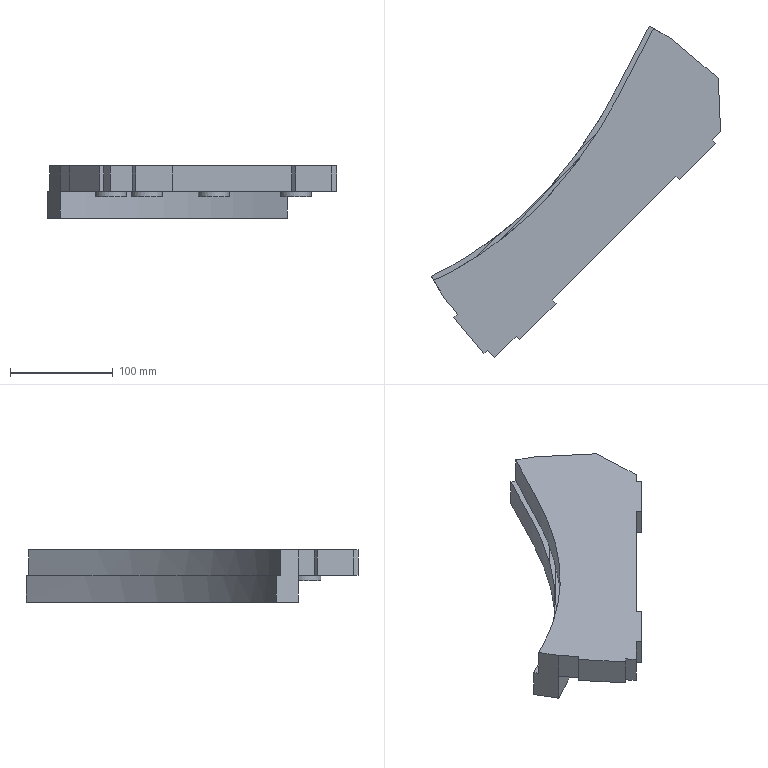Part | NX | features solid 2 | 1 solid | 38 faces | box 281.55 x 323.19 x 51 mm | volume 976674 mm3 | plane 29 | cylinder 5 | spline 4 | commonest cylinder face diameters 30 x5
STEP:
#1=CARTESIAN_POINT('',(378.604,-622.777,20.));
#2=VERTEX_POINT('',#1);
#3=CARTESIAN_POINT('',(378.604,-622.777,45.));
#4=VERTEX_POINT('',#3);
#5=CARTESIAN_POINT('',(378.604,-622.777,20.));
#6=DIRECTION('',(0.,0.,1.));
#7=VECTOR('',#6,1000.);
#8=LINE('',#5,#7);
#9=EDGE_CURVE('',#2,#4,#8,.T.);
#10=ORIENTED_EDGE('',*,*,#9,.F.);
#11=CARTESIAN_POINT('',(385.032,-630.437,20.));
#12=VERTEX_POINT('',#11);
#13=CARTESIAN_POINT('',(339.027,-575.611,20.));
#14=DIRECTION('',(-0.6428,0.766,0.));
#15=VECTOR('',#14,1000.);
#16=LINE('',#13,#15);
#17=EDGE_CURVE('',#12,#2,#16,.T.);
#18=ORIENTED_EDGE('',*,*,#17,.F.);
#19=CARTESIAN_POINT('',(385.032,-630.437,45.));
#20=VERTEX_POINT('',#19);
#21=CARTESIAN_POINT('',(385.032,-630.437,45.));
#22=DIRECTION('',(0.,0.,1.));
#23=VECTOR('',#22,1000.);
#24=LINE('',#21,#23);
#25=EDGE_CURVE('',#12,#20,#24,.T.);
#26=ORIENTED_EDGE('',*,*,#25,.T.);
#27=CARTESIAN_POINT('',(323.293,-556.86,45.));
#28=DIRECTION('',(0.6428,-0.766,0.));
#29=VECTOR('',#28,1000.);
#30=LINE('',#27,#29);
#31=EDGE_CURVE('',#4,#20,#30,.T.);
#32=ORIENTED_EDGE('',*,*,#31,.F.);
#33=EDGE_LOOP('',(#10,#18,#26,#32));
#34=FACE_BOUND('',#33,.T.);
#35=CARTESIAN_POINT('',(389.886,-636.222,20.));
#36=DIRECTION('',(0.766,0.6428,0.));
#37=DIRECTION('',(-0.6428,0.766,0.));
#38=AXIS2_PLACEMENT_3D('',#35,#36,#37);
#39=PLANE('',#38);
#40=ADVANCED_FACE('',(#34),#39,.F.);
#41=CARTESIAN_POINT('',(349.161,-587.688,45.));
#42=VERTEX_POINT('',#41);
#43=CARTESIAN_POINT('',(349.161,-587.688,20.));
#44=VERTEX_POINT('',#43);
#45=CARTESIAN_POINT('',(349.161,-587.688,20.));
#46=DIRECTION('',(0.,0.,-1.));
#47=VECTOR('',#46,1000.);
#48=LINE('',#45,#47);
#49=EDGE_CURVE('',#42,#44,#48,.T.);
#50=ORIENTED_EDGE('',*,*,#49,.F.);
#51=CARTESIAN_POINT('',(336.306,-572.367,45.));
#52=VERTEX_POINT('',#51);
#53=CARTESIAN_POINT('',(323.293,-556.86,45.));
#54=DIRECTION('',(0.6428,-0.766,0.));
#55=VECTOR('',#54,1000.);
#56=LINE('',#53,#55);
#57=EDGE_CURVE('',#52,#42,#56,.T.);
#58=ORIENTED_EDGE('',*,*,#57,.F.);
#59=CARTESIAN_POINT('',(336.306,-572.367,20.));
#60=VERTEX_POINT('',#59);
#61=CARTESIAN_POINT('',(336.306,-572.367,45.));
#62=DIRECTION('',(0.,0.,-1.));
#63=VECTOR('',#62,1000.);
#64=LINE('',#61,#63);
#65=EDGE_CURVE('',#52,#60,#64,.T.);
#66=ORIENTED_EDGE('',*,*,#65,.T.);
#67=CARTESIAN_POINT('',(339.027,-575.611,20.));
#68=DIRECTION('',(-0.6428,0.766,0.));
#69=VECTOR('',#68,1000.);
#70=LINE('',#67,#69);
#71=EDGE_CURVE('',#44,#60,#70,.T.);
#72=ORIENTED_EDGE('',*,*,#71,.F.);
#73=EDGE_LOOP('',(#50,#58,#66,#72));
#74=FACE_BOUND('',#73,.T.);
#75=CARTESIAN_POINT('',(389.886,-636.222,20.));
#76=DIRECTION('',(0.766,0.6428,0.));
#77=DIRECTION('',(-0.6428,0.766,0.));
#78=AXIS2_PLACEMENT_3D('',#75,#76,#77);
#79=PLANE('',#78);
#80=ADVANCED_FACE('',(#74),#79,.F.);
#81=CARTESIAN_POINT('',(445.136,-577.404,20.));
#82=VERTEX_POINT('',#81);
#83=CARTESIAN_POINT('',(441.601,-573.869,20.));
#84=VERTEX_POINT('',#83);
#85=CARTESIAN_POINT('',(445.136,-577.404,20.));
#86=DIRECTION('',(-0.7071,0.7071,0.));
#87=VECTOR('',#86,1000.);
#88=LINE('',#85,#87);
#89=EDGE_CURVE('',#82,#84,#88,.T.);
#90=ORIENTED_EDGE('',*,*,#89,.F.);
#91=CARTESIAN_POINT('',(409.781,-612.76,20.));
#92=VERTEX_POINT('',#91);
#93=CARTESIAN_POINT('',(649.557,-372.983,20.));
#94=DIRECTION('',(-0.7071,-0.7071,0.));
#95=VECTOR('',#94,1000.);
#96=LINE('',#93,#95);
#97=EDGE_CURVE('',#82,#92,#96,.T.);
#98=ORIENTED_EDGE('',*,*,#97,.T.);
#99=CARTESIAN_POINT('',(406.245,-609.224,20.));
#100=VERTEX_POINT('',#99);
#101=CARTESIAN_POINT('',(409.781,-612.76,20.));
#102=DIRECTION('',(-0.7071,0.7071,0.));
#103=VECTOR('',#102,1000.);
#104=LINE('',#101,#103);
#105=EDGE_CURVE('',#92,#100,#104,.T.);
#106=ORIENTED_EDGE('',*,*,#105,.T.);
#107=CARTESIAN_POINT('',(646.022,-369.447,20.));
#108=DIRECTION('',(-0.7071,-0.7071,0.));
#109=VECTOR('',#108,1000.);
#110=LINE('',#107,#109);
#111=EDGE_CURVE('',#100,#12,#110,.T.);
#112=ORIENTED_EDGE('',*,*,#111,.T.);
#113=ORIENTED_EDGE('',*,*,#17,.T.);
#114=CARTESIAN_POINT('',(374.774,-625.991,20.));
#115=VERTEX_POINT('',#114);
#116=CARTESIAN_POINT('',(374.774,-625.991,20.));
#117=DIRECTION('',(0.766,0.6428,0.));
#118=VECTOR('',#117,1000.);
#119=LINE('',#116,#118);
#120=EDGE_CURVE('',#115,#2,#119,.T.);
#121=ORIENTED_EDGE('',*,*,#120,.F.);
#122=CARTESIAN_POINT('',(345.331,-590.902,20.));
#123=VERTEX_POINT('',#122);
#124=CARTESIAN_POINT('',(335.197,-578.825,20.));
#125=DIRECTION('',(-0.6428,0.766,0.));
#126=VECTOR('',#125,1000.);
#127=LINE('',#124,#126);
#128=EDGE_CURVE('',#115,#123,#127,.T.);
#129=ORIENTED_EDGE('',*,*,#128,.T.);
#130=CARTESIAN_POINT('',(345.331,-590.902,20.));
#131=DIRECTION('',(0.766,0.6428,0.));
#132=VECTOR('',#131,1000.);
#133=LINE('',#130,#132);
#134=EDGE_CURVE('',#123,#44,#133,.T.);
#135=ORIENTED_EDGE('',*,*,#134,.T.);
#136=ORIENTED_EDGE('',*,*,#71,.T.);
#137=CARTESIAN_POINT('',(557.374,-319.761,20.));
#138=VERTEX_POINT('',#137);
#139=CARTESIAN_POINT('',(557.374,-319.761,20.));
#140=CARTESIAN_POINT('',(551.234,-331.629,20.));
#141=CARTESIAN_POINT('',(541.911,-349.627,20.));
#142=CARTESIAN_POINT('',(531.108,-370.579,20.));
#143=CARTESIAN_POINT('',(524.631,-383.018,20.));
#144=CARTESIAN_POINT('',(514.348,-402.01,20.));
#145=CARTESIAN_POINT('',(497.659,-429.783,20.));
#146=CARTESIAN_POINT('',(471.931,-465.101,20.));
#147=CARTESIAN_POINT('',(442.6,-497.853,20.));
#148=CARTESIAN_POINT('',(409.743,-527.289,20.));
#149=CARTESIAN_POINT('',(379.681,-548.594,20.));
#150=CARTESIAN_POINT('',(357.354,-561.599,20.));
#151=CARTESIAN_POINT('',(346.037,-567.559,20.));
#152=CARTESIAN_POINT('',(339.912,-570.613,20.));
#153=CARTESIAN_POINT('',(337.327,-571.87,20.));
#154=CARTESIAN_POINT('',(336.306,-572.367,20.));
#155=B_SPLINE_CURVE_WITH_KNOTS('',3,(#139,#140,#141,#142,#143,#144,#145,#146,#147,#148,#149,#150,#151,#152,#153,#154),.UNSPECIFIED.,.F.,.F.,(4,1,1,1,1,1,1,1,1,1,1,1,1,4),(0.,0.1226,0.1856,0.2172,0.2487,0.3748,0.5009,0.627,0.7531,0.8792,0.9423,0.9738,0.9896,1.),.UNSPECIFIED.);
#156=EDGE_CURVE('',#138,#60,#155,.T.);
#157=ORIENTED_EDGE('',*,*,#156,.F.);
#158=CARTESIAN_POINT('',(603.051,-358.089,20.));
#159=VERTEX_POINT('',#158);
#160=CARTESIAN_POINT('',(578.233,-337.263,20.));
#161=DIRECTION('',(-0.766,0.6428,0.));
#162=VECTOR('',#161,1000.);
#163=LINE('',#160,#162);
#164=EDGE_CURVE('',#159,#138,#163,.T.);
#165=ORIENTED_EDGE('',*,*,#164,.F.);
#166=CARTESIAN_POINT('',(605.324,-410.145,20.));
#167=VERTEX_POINT('',#166);
#168=CARTESIAN_POINT('',(604.924,-400.991,20.));
#169=DIRECTION('',(-0.04362,0.999,0.));
#170=VECTOR('',#169,1000.);
#171=LINE('',#168,#170);
#172=EDGE_CURVE('',#159,#167,#171,.F.);
#173=ORIENTED_EDGE('',*,*,#172,.T.);
#174=CARTESIAN_POINT('',(597.237,-418.232,20.));
#175=VERTEX_POINT('',#174);
#176=CARTESIAN_POINT('',(646.022,-369.447,20.));
#177=DIRECTION('',(-0.7071,-0.7071,0.));
#178=VECTOR('',#177,1000.);
#179=LINE('',#176,#178);
#180=EDGE_CURVE('',#167,#175,#179,.T.);
#181=ORIENTED_EDGE('',*,*,#180,.T.);
#182=CARTESIAN_POINT('',(600.773,-421.768,20.));
#183=VERTEX_POINT('',#182);
#184=CARTESIAN_POINT('',(600.773,-421.768,20.));
#185=DIRECTION('',(-0.7071,0.7071,0.));
#186=VECTOR('',#185,1000.);
#187=LINE('',#184,#186);
#188=EDGE_CURVE('',#183,#175,#187,.T.);
#189=ORIENTED_EDGE('',*,*,#188,.F.);
#190=CARTESIAN_POINT('',(565.417,-457.123,20.));
#191=VERTEX_POINT('',#190);
#192=CARTESIAN_POINT('',(840.549,-181.991,20.));
#193=DIRECTION('',(-0.7071,-0.7071,0.));
#194=VECTOR('',#193,1000.);
#195=LINE('',#192,#194);
#196=EDGE_CURVE('',#183,#191,#195,.T.);
#197=ORIENTED_EDGE('',*,*,#196,.T.);
#198=CARTESIAN_POINT('',(561.882,-453.587,20.));
#199=VERTEX_POINT('',#198);
#200=CARTESIAN_POINT('',(565.417,-457.123,20.));
#201=DIRECTION('',(-0.7071,0.7071,0.));
#202=VECTOR('',#201,1000.);
#203=LINE('',#200,#202);
#204=EDGE_CURVE('',#191,#199,#203,.T.);
#205=ORIENTED_EDGE('',*,*,#204,.T.);
#206=CARTESIAN_POINT('',(646.022,-369.447,20.));
#207=DIRECTION('',(-0.7071,-0.7071,0.));
#208=VECTOR('',#207,1000.);
#209=LINE('',#206,#208);
#210=EDGE_CURVE('',#199,#84,#209,.T.);
#211=ORIENTED_EDGE('',*,*,#210,.T.);
#212=EDGE_LOOP('',(#90,#98,#106,#112,#113,#121,#129,#135,#136,#157,#165,#173,#181,#189,#197,#205,#211));
#213=FACE_BOUND('',#212,.T.);
#214=CARTESIAN_POINT('',(500.617,-484.28,20.));
#215=VERTEX_POINT('',#214);
#216=CARTESIAN_POINT('',(485.617,-484.28,20.));
#217=DIRECTION('',(0.,0.,1.));
#218=DIRECTION('',(1.,0.,0.));
#219=AXIS2_PLACEMENT_3D('',#216,#217,#218);
#220=CIRCLE('',#219,15.);
#221=EDGE_CURVE('',#215,#215,#220,.F.);
#222=ORIENTED_EDGE('',*,*,#221,.F.);
#223=EDGE_LOOP('',(#222));
#224=FACE_BOUND('',#223,.T.);
#225=CARTESIAN_POINT('',(400.617,-579.28,20.));
#226=VERTEX_POINT('',#225);
#227=CARTESIAN_POINT('',(385.617,-579.28,20.));
#228=DIRECTION('',(0.,0.,1.));
#229=DIRECTION('',(1.,0.,0.));
#230=AXIS2_PLACEMENT_3D('',#227,#228,#229);
#231=CIRCLE('',#230,15.);
#232=EDGE_CURVE('',#226,#226,#231,.F.);
#233=ORIENTED_EDGE('',*,*,#232,.F.);
#234=EDGE_LOOP('',(#233));
#235=FACE_BOUND('',#234,.T.);
#236=CARTESIAN_POINT('',(435.617,-564.28,20.));
#237=VERTEX_POINT('',#236);
#238=CARTESIAN_POINT('',(420.617,-564.28,20.));
#239=DIRECTION('',(0.,0.,1.));
#240=DIRECTION('',(1.,0.,0.));
#241=AXIS2_PLACEMENT_3D('',#238,#239,#240);
#242=CIRCLE('',#241,15.);
#243=EDGE_CURVE('',#237,#237,#242,.F.);
#244=ORIENTED_EDGE('',*,*,#243,.F.);
#245=EDGE_LOOP('',(#244));
#246=FACE_BOUND('',#245,.T.);
#247=CARTESIAN_POINT('',(580.617,-414.28,20.));
#248=VERTEX_POINT('',#247);
#249=CARTESIAN_POINT('',(565.617,-414.28,20.));
#250=DIRECTION('',(0.,0.,1.));
#251=DIRECTION('',(1.,0.,0.));
#252=AXIS2_PLACEMENT_3D('',#249,#250,#251);
#253=CIRCLE('',#252,15.);
#254=EDGE_CURVE('',#248,#248,#253,.F.);
#255=ORIENTED_EDGE('',*,*,#254,.F.);
#256=EDGE_LOOP('',(#255));
#257=FACE_BOUND('',#256,.T.);
#258=CARTESIAN_POINT('',(580.617,-374.28,20.));
#259=VERTEX_POINT('',#258);
#260=CARTESIAN_POINT('',(565.617,-374.28,20.));
#261=DIRECTION('',(0.,0.,1.));
#262=DIRECTION('',(1.,0.,0.));
#263=AXIS2_PLACEMENT_3D('',#260,#261,#262);
#264=CIRCLE('',#263,15.);
#265=EDGE_CURVE('',#259,#259,#264,.F.);
#266=ORIENTED_EDGE('',*,*,#265,.F.);
#267=EDGE_LOOP('',(#266));
#268=FACE_BOUND('',#267,.T.);
#269=CARTESIAN_POINT('',(389.043,-612.022,20.));
#270=DIRECTION('',(0.,0.,-1.));
#271=DIRECTION('',(-1.,0.,0.));
#272=AXIS2_PLACEMENT_3D('',#269,#270,#271);
#273=PLANE('',#272);
#274=ADVANCED_FACE('',(#213,#224,#235,#246,#257,#268),#273,.T.);
#275=CARTESIAN_POINT('',(557.374,-319.761,-6.));
#276=VERTEX_POINT('',#275);
#277=CARTESIAN_POINT('',(535.7,-307.247,-6.));
#278=VERTEX_POINT('',#277);
#279=CARTESIAN_POINT('',(557.374,-319.761,-6.));
#280=DIRECTION('',(-0.866,0.5,0.));
#281=VECTOR('',#280,1000.);
#282=LINE('',#279,#281);
#283=EDGE_CURVE('',#276,#278,#282,.T.);
#284=ORIENTED_EDGE('',*,*,#283,.F.);
#285=CARTESIAN_POINT('',(336.306,-572.367,-6.));
#286=VERTEX_POINT('',#285);
#287=CARTESIAN_POINT('',(557.374,-319.761,-6.));
#288=CARTESIAN_POINT('',(551.234,-331.629,-6.));
#289=CARTESIAN_POINT('',(541.911,-349.627,-6.));
#290=CARTESIAN_POINT('',(531.108,-370.579,-6.));
#291=CARTESIAN_POINT('',(524.631,-383.018,-6.));
#292=CARTESIAN_POINT('',(514.348,-402.01,-6.));
#293=CARTESIAN_POINT('',(497.659,-429.783,-6.));
#294=CARTESIAN_POINT('',(471.931,-465.101,-6.));
#295=CARTESIAN_POINT('',(442.6,-497.853,-6.));
#296=CARTESIAN_POINT('',(409.743,-527.289,-6.));
#297=CARTESIAN_POINT('',(379.681,-548.594,-6.));
#298=CARTESIAN_POINT('',(357.354,-561.599,-6.));
#299=CARTESIAN_POINT('',(346.037,-567.559,-6.));
#300=CARTESIAN_POINT('',(339.912,-570.613,-6.));
#301=CARTESIAN_POINT('',(337.327,-571.87,-6.));
#302=CARTESIAN_POINT('',(336.306,-572.367,-6.));
#303=B_SPLINE_CURVE_WITH_KNOTS('',3,(#287,#288,#289,#290,#291,#292,#293,#294,#295,#296,#297,#298,#299,#300,#301,#302),.UNSPECIFIED.,.F.,.F.,(4,1,1,1,1,1,1,1,1,1,1,1,1,4),(0.,0.1226,0.1856,0.2172,0.2487,0.3748,0.5009,0.627,0.7531,0.8792,0.9423,0.9738,0.9896,1.),.UNSPECIFIED.);
#304=EDGE_CURVE('',#276,#286,#303,.T.);
#305=ORIENTED_EDGE('',*,*,#304,.T.);
#306=CARTESIAN_POINT('',(323.774,-550.663,-6.));
#307=VERTEX_POINT('',#306);
#308=CARTESIAN_POINT('',(336.306,-572.367,-6.));
#309=DIRECTION('',(-0.5,0.866,0.));
#310=VECTOR('',#309,1000.);
#311=LINE('',#308,#310);
#312=EDGE_CURVE('',#286,#307,#311,.T.);
#313=ORIENTED_EDGE('',*,*,#312,.T.);
#314=CARTESIAN_POINT('',(535.7,-307.247,-6.));
#315=CARTESIAN_POINT('',(534.934,-308.728,-6.));
#316=CARTESIAN_POINT('',(529.574,-319.09,-6.));
#317=CARTESIAN_POINT('',(521.917,-333.894,-6.));
#318=CARTESIAN_POINT('',(512.728,-351.658,-6.));
#319=CARTESIAN_POINT('',(506.903,-362.951,-6.));
#320=CARTESIAN_POINT('',(499.555,-376.977,-6.));
#321=CARTESIAN_POINT('',(488.977,-395.893,-6.));
#322=CARTESIAN_POINT('',(467.289,-430.253,-6.));
#323=CARTESIAN_POINT('',(433.523,-472.816,-6.));
#324=CARTESIAN_POINT('',(392.995,-509.066,-6.));
#325=CARTESIAN_POINT('',(357.027,-533.308,-6.));
#326=CARTESIAN_POINT('',(337.263,-544.104,-6.));
#327=CARTESIAN_POINT('',(326.021,-549.566,-6.));
#328=CARTESIAN_POINT('',(324.523,-550.297,-6.));
#329=CARTESIAN_POINT('',(323.774,-550.663,-6.));
#330=B_SPLINE_CURVE_WITH_KNOTS('',3,(#314,#315,#316,#317,#318,#319,#320,#321,#322,#323,#324,#325,#326,#327,#328,#329),.UNSPECIFIED.,.F.,.F.,(4,1,1,1,1,1,1,1,1,1,1,1,1,4),(0.,0.01516,0.1061,0.1516,0.197,0.2216,0.2955,0.394,0.5909,0.7879,0.8864,0.9848,0.9924,1.),.UNSPECIFIED.);
#331=EDGE_CURVE('',#278,#307,#330,.T.);
#332=ORIENTED_EDGE('',*,*,#331,.F.);
#333=EDGE_LOOP('',(#284,#305,#313,#332));
#334=FACE_BOUND('',#333,.T.);
#335=CARTESIAN_POINT('',(631.984,-1285.265,-6.));
#336=DIRECTION('',(0.,0.,1.));
#337=DIRECTION('',(1.,0.,0.));
#338=AXIS2_PLACEMENT_3D('',#335,#336,#337);
#339=PLANE('',#338);
#340=ADVANCED_FACE('',(#334),#339,.F.);
#341=CARTESIAN_POINT('',(435.617,-564.28,15.));
#342=VERTEX_POINT('',#341);
#343=CARTESIAN_POINT('',(420.617,-564.28,15.));
#344=DIRECTION('',(0.,0.,1.));
#345=DIRECTION('',(1.,0.,0.));
#346=AXIS2_PLACEMENT_3D('',#343,#344,#345);
#347=CIRCLE('',#346,15.);
#348=EDGE_CURVE('',#342,#342,#347,.T.);
#349=ORIENTED_EDGE('',*,*,#348,.F.);
#350=EDGE_LOOP('',(#349));
#351=FACE_BOUND('',#350,.T.);
#352=CARTESIAN_POINT('',(425.617,-559.28,15.));
#353=DIRECTION('',(0.,0.,1.));
#354=DIRECTION('',(1.,0.,0.));
#355=AXIS2_PLACEMENT_3D('',#352,#353,#354);
#356=PLANE('',#355);
#357=ADVANCED_FACE('',(#351),#356,.F.);
#358=CARTESIAN_POINT('',(580.617,-414.28,15.));
#359=VERTEX_POINT('',#358);
#360=CARTESIAN_POINT('',(565.617,-414.28,15.));
#361=DIRECTION('',(0.,0.,1.));
#362=DIRECTION('',(1.,0.,0.));
#363=AXIS2_PLACEMENT_3D('',#360,#361,#362);
#364=CIRCLE('',#363,15.);
#365=EDGE_CURVE('',#359,#359,#364,.T.);
#366=ORIENTED_EDGE('',*,*,#365,.F.);
#367=EDGE_LOOP('',(#366));
#368=FACE_BOUND('',#367,.T.);
#369=CARTESIAN_POINT('',(545.617,-419.28,15.));
#370=DIRECTION('',(0.,0.,1.));
#371=DIRECTION('',(1.,0.,0.));
#372=AXIS2_PLACEMENT_3D('',#369,#370,#371);
#373=PLANE('',#372);
#374=ADVANCED_FACE('',(#368),#373,.F.);
#375=CARTESIAN_POINT('',(500.617,-484.28,15.));
#376=VERTEX_POINT('',#375);
#377=CARTESIAN_POINT('',(485.617,-484.28,15.));
#378=DIRECTION('',(0.,0.,1.));
#379=DIRECTION('',(1.,0.,0.));
#380=AXIS2_PLACEMENT_3D('',#377,#378,#379);
#381=CIRCLE('',#380,15.);
#382=EDGE_CURVE('',#376,#376,#381,.T.);
#383=ORIENTED_EDGE('',*,*,#382,.F.);
#384=EDGE_LOOP('',(#383));
#385=FACE_BOUND('',#384,.T.);
#386=CARTESIAN_POINT('',(465.617,-504.28,15.));
#387=DIRECTION('',(0.,0.,1.));
#388=DIRECTION('',(1.,0.,0.));
#389=AXIS2_PLACEMENT_3D('',#386,#387,#388);
#390=PLANE('',#389);
#391=ADVANCED_FACE('',(#385),#390,.F.);
#392=CARTESIAN_POINT('',(400.617,-579.28,15.));
#393=VERTEX_POINT('',#392);
#394=CARTESIAN_POINT('',(385.617,-579.28,15.));
#395=DIRECTION('',(0.,0.,1.));
#396=DIRECTION('',(1.,0.,0.));
#397=AXIS2_PLACEMENT_3D('',#394,#395,#396);
#398=CIRCLE('',#397,15.);
#399=EDGE_CURVE('',#393,#393,#398,.T.);
#400=ORIENTED_EDGE('',*,*,#399,.F.);
#401=EDGE_LOOP('',(#400));
#402=FACE_BOUND('',#401,.T.);
#403=CARTESIAN_POINT('',(390.617,-574.28,15.));
#404=DIRECTION('',(0.,0.,1.));
#405=DIRECTION('',(1.,0.,0.));
#406=AXIS2_PLACEMENT_3D('',#403,#404,#405);
#407=PLANE('',#406);
#408=ADVANCED_FACE('',(#402),#407,.F.);
#409=CARTESIAN_POINT('',(445.136,-577.404,45.));
#410=VERTEX_POINT('',#409);
#411=CARTESIAN_POINT('',(409.781,-612.76,45.));
#412=VERTEX_POINT('',#411);
#413=CARTESIAN_POINT('',(512.74,-509.801,45.));
#414=DIRECTION('',(-0.7071,-0.7071,0.));
#415=VECTOR('',#414,1000.);
#416=LINE('',#413,#415);
#417=EDGE_CURVE('',#410,#412,#416,.T.);
#418=ORIENTED_EDGE('',*,*,#417,.F.);
#419=CARTESIAN_POINT('',(441.601,-573.869,45.));
#420=VERTEX_POINT('',#419);
#421=CARTESIAN_POINT('',(445.136,-577.404,45.));
#422=DIRECTION('',(-0.7071,0.7071,0.));
#423=VECTOR('',#422,1000.);
#424=LINE('',#421,#423);
#425=EDGE_CURVE('',#410,#420,#424,.T.);
#426=ORIENTED_EDGE('',*,*,#425,.T.);
#427=CARTESIAN_POINT('',(561.882,-453.587,45.));
#428=VERTEX_POINT('',#427);
#429=CARTESIAN_POINT('',(509.204,-506.265,45.));
#430=DIRECTION('',(-0.7071,-0.7071,0.));
#431=VECTOR('',#430,1000.);
#432=LINE('',#429,#431);
#433=EDGE_CURVE('',#428,#420,#432,.T.);
#434=ORIENTED_EDGE('',*,*,#433,.F.);
#435=CARTESIAN_POINT('',(565.417,-457.123,45.));
#436=VERTEX_POINT('',#435);
#437=CARTESIAN_POINT('',(565.417,-457.123,45.));
#438=DIRECTION('',(-0.7071,0.7071,0.));
#439=VECTOR('',#438,1000.);
#440=LINE('',#437,#439);
#441=EDGE_CURVE('',#436,#428,#440,.T.);
#442=ORIENTED_EDGE('',*,*,#441,.F.);
#443=CARTESIAN_POINT('',(600.773,-421.768,45.));
#444=VERTEX_POINT('',#443);
#445=CARTESIAN_POINT('',(703.732,-318.809,45.));
#446=DIRECTION('',(-0.7071,-0.7071,0.));
#447=VECTOR('',#446,1000.);
#448=LINE('',#445,#447);
#449=EDGE_CURVE('',#444,#436,#448,.T.);
#450=ORIENTED_EDGE('',*,*,#449,.F.);
#451=CARTESIAN_POINT('',(597.237,-418.232,45.));
#452=VERTEX_POINT('',#451);
#453=CARTESIAN_POINT('',(600.773,-421.768,45.));
#454=DIRECTION('',(-0.7071,0.7071,0.));
#455=VECTOR('',#454,1000.);
#456=LINE('',#453,#455);
#457=EDGE_CURVE('',#444,#452,#456,.T.);
#458=ORIENTED_EDGE('',*,*,#457,.T.);
#459=CARTESIAN_POINT('',(605.324,-410.145,45.));
#460=VERTEX_POINT('',#459);
#461=CARTESIAN_POINT('',(509.204,-506.265,45.));
#462=DIRECTION('',(-0.7071,-0.7071,0.));
#463=VECTOR('',#462,1000.);
#464=LINE('',#461,#463);
#465=EDGE_CURVE('',#460,#452,#464,.T.);
#466=ORIENTED_EDGE('',*,*,#465,.F.);
#467=CARTESIAN_POINT('',(603.051,-358.089,45.));
#468=VERTEX_POINT('',#467);
#469=CARTESIAN_POINT('',(604.924,-400.991,45.));
#470=DIRECTION('',(0.04362,-0.999,0.));
#471=VECTOR('',#470,1000.);
#472=LINE('',#469,#471);
#473=EDGE_CURVE('',#460,#468,#472,.F.);
#474=ORIENTED_EDGE('',*,*,#473,.T.);
#475=CARTESIAN_POINT('',(557.374,-319.761,45.));
#476=VERTEX_POINT('',#475);
#477=CARTESIAN_POINT('',(559.089,-321.2,45.));
#478=DIRECTION('',(0.766,-0.6428,0.));
#479=VECTOR('',#478,1000.);
#480=LINE('',#477,#479);
#481=EDGE_CURVE('',#476,#468,#480,.T.);
#482=ORIENTED_EDGE('',*,*,#481,.F.);
#483=CARTESIAN_POINT('',(540.035,-309.75,45.));
#484=VERTEX_POINT('',#483);
#485=CARTESIAN_POINT('',(557.374,-319.761,45.));
#486=DIRECTION('',(-0.866,0.5,0.));
#487=VECTOR('',#486,1000.);
#488=LINE('',#485,#487);
#489=EDGE_CURVE('',#476,#484,#488,.T.);
#490=ORIENTED_EDGE('',*,*,#489,.T.);
#491=CARTESIAN_POINT('',(326.28,-555.003,45.));
#492=VERTEX_POINT('',#491);
#493=CARTESIAN_POINT('',(540.035,-309.75,45.));
#494=CARTESIAN_POINT('',(537.021,-315.576,45.));
#495=CARTESIAN_POINT('',(533.033,-323.285,45.));
#496=CARTESIAN_POINT('',(528.78,-331.507,45.));
#497=CARTESIAN_POINT('',(526.123,-336.645,45.));
#498=CARTESIAN_POINT('',(524.351,-340.07,45.));
#499=CARTESIAN_POINT('',(523.2,-342.295,45.));
#500=CARTESIAN_POINT('',(522.47,-343.707,45.));
#501=CARTESIAN_POINT('',(521.972,-344.669,45.));
#502=CARTESIAN_POINT('',(521.641,-345.31,45.));
#503=CARTESIAN_POINT('',(521.425,-345.727,45.));
#504=CARTESIAN_POINT('',(521.243,-346.079,45.));
#505=CARTESIAN_POINT('',(521.119,-346.319,45.));
#506=CARTESIAN_POINT('',(521.036,-346.479,45.));
#507=CARTESIAN_POINT('',(520.992,-346.565,45.));
#508=CARTESIAN_POINT('',(520.96,-346.627,45.));
#509=CARTESIAN_POINT('',(520.939,-346.667,45.));
#510=CARTESIAN_POINT('',(520.92,-346.704,45.));
#511=CARTESIAN_POINT('',(520.914,-346.714,45.));
#512=CARTESIAN_POINT('',(520.9,-346.742,45.));
#513=CARTESIAN_POINT('',(520.922,-346.7,45.));
#514=CARTESIAN_POINT('',(520.822,-346.893,45.));
#515=CARTESIAN_POINT('',(520.731,-347.068,45.));
#516=CARTESIAN_POINT('',(520.554,-347.411,45.));
#517=CARTESIAN_POINT('',(520.315,-347.874,45.));
#518=CARTESIAN_POINT('',(520.028,-348.429,45.));
#519=CARTESIAN_POINT('',(519.652,-349.155,45.));
#520=CARTESIAN_POINT('',(519.194,-350.041,45.));
#521=CARTESIAN_POINT('',(518.487,-351.409,45.));
#522=CARTESIAN_POINT('',(517.648,-353.031,45.));
#523=CARTESIAN_POINT('',(516.716,-354.833,45.));
#524=CARTESIAN_POINT('',(515.859,-356.491,45.));
#525=CARTESIAN_POINT('',(514.814,-358.511,45.));
#526=CARTESIAN_POINT('',(513.694,-360.677,45.));
#527=CARTESIAN_POINT('',(512.647,-362.702,45.));
#528=CARTESIAN_POINT('',(512.022,-363.91,45.));
#529=CARTESIAN_POINT('',(511.67,-364.592,45.));
#530=CARTESIAN_POINT('',(511.514,-364.893,45.));
#531=CARTESIAN_POINT('',(511.421,-365.073,45.));
#532=CARTESIAN_POINT('',(511.385,-365.143,45.));
#533=CARTESIAN_POINT('',(511.309,-365.29,45.));
#534=CARTESIAN_POINT('',(511.443,-365.031,45.));
#535=CARTESIAN_POINT('',(511.152,-365.592,45.));
#536=CARTESIAN_POINT('',(510.931,-366.015,45.));
#537=CARTESIAN_POINT('',(510.634,-366.587,45.));
#538=CARTESIAN_POINT('',(510.29,-367.247,45.));
#539=CARTESIAN_POINT('',(509.831,-368.124,45.));
#540=CARTESIAN_POINT('',(509.267,-369.202,45.));
#541=CARTESIAN_POINT('',(508.379,-370.892,45.));
#542=CARTESIAN_POINT('',(507.298,-372.939,45.));
#543=CARTESIAN_POINT('',(505.633,-376.069,45.));
#544=CARTESIAN_POINT('',(504.056,-378.996,45.));
#545=CARTESIAN_POINT('',(502.773,-381.345,45.));
#546=CARTESIAN_POINT('',(502.041,-382.674,45.));
#547=CARTESIAN_POINT('',(501.566,-383.53,45.));
#548=CARTESIAN_POINT('',(500.863,-384.793,45.));
#549=CARTESIAN_POINT('',(500.003,-386.328,45.));
#550=CARTESIAN_POINT('',(498.456,-389.067,45.));
#551=CARTESIAN_POINT('',(496.253,-392.904,45.));
#552=CARTESIAN_POINT('',(493.579,-397.458,45.));
#553=CARTESIAN_POINT('',(489.987,-403.439,45.));
#554=CARTESIAN_POINT('',(486.36,-409.279,45.));
#555=CARTESIAN_POINT('',(482.666,-415.023,45.));
#556=CARTESIAN_POINT('',(479.938,-419.17,45.));
#557=CARTESIAN_POINT('',(476.943,-423.616,45.));
#558=CARTESIAN_POINT('',(472.985,-429.346,45.));
#559=CARTESIAN_POINT('',(467.919,-436.415,45.));
#560=CARTESIAN_POINT('',(462.756,-443.27,45.));
#561=CARTESIAN_POINT('',(458.532,-448.672,45.));
#562=CARTESIAN_POINT('',(455.389,-452.596,45.));
#563=CARTESIAN_POINT('',(451.985,-456.738,45.));
#564=CARTESIAN_POINT('',(447.469,-462.087,45.));
#565=CARTESIAN_POINT('',(439.39,-471.287,45.));
#566=CARTESIAN_POINT('',(427.458,-483.827,45.));
#567=CARTESIAN_POINT('',(414.999,-495.585,45.));
#568=CARTESIAN_POINT('',(404.673,-504.551,45.));
#569=CARTESIAN_POINT('',(396.866,-510.966,45.));
#570=CARTESIAN_POINT('',(388.52,-517.44,45.));
#571=CARTESIAN_POINT('',(380.122,-523.568,45.));
#572=CARTESIAN_POINT('',(371.544,-529.457,45.));
#573=CARTESIAN_POINT('',(362.813,-535.083,45.));
#574=CARTESIAN_POINT('',(355.426,-539.543,45.));
#575=CARTESIAN_POINT('',(349.414,-542.997,45.));
#576=CARTESIAN_POINT('',(345.604,-545.113,45.));
#577=CARTESIAN_POINT('',(342.562,-546.759,45.));
#578=CARTESIAN_POINT('',(340.262,-547.983,45.));
#579=CARTESIAN_POINT('',(338.348,-548.984,45.));
#580=CARTESIAN_POINT('',(336.98,-549.691,45.));
#581=CARTESIAN_POINT('',(336.233,-550.074,45.));
#582=CARTESIAN_POINT('',(335.57,-550.412,45.));
#583=CARTESIAN_POINT('',(335.294,-550.553,45.));
#584=CARTESIAN_POINT('',(334.741,-550.832,45.));
#585=CARTESIAN_POINT('',(334.026,-551.191,45.));
#586=CARTESIAN_POINT('',(333.029,-551.688,45.));
#587=CARTESIAN_POINT('',(331.55,-552.421,45.));
#588=CARTESIAN_POINT('',(329.404,-553.477,45.));
#589=CARTESIAN_POINT('',(327.374,-554.47,45.));
#590=CARTESIAN_POINT('',(326.28,-555.003,45.));
#591=B_SPLINE_CURVE_WITH_KNOTS('',3,(#493,#494,#495,#496,#497,#498,#499,#500,#501,#502,#503,#504,#505,#506,#507,#508,#509,#510,#511,#512,#513,#514,#515,#516,#517,#518,#519,#520,#521,#522,#523,#524,#525,#526,#527,#528,#529,#530,#531,#532,#533,#534,#535,#536,#537,#538,#539,#540,#541,#542,#543,#544,#545,#546,#547,#548,#549,#550,#551,#552,#553,#554,#555,#556,#557,#558,#559,#560,#561,#562,#563,#564,#565,#566,#567,#568,#569,#570,#571,#572,#573,#574,#575,#576,#577,#578,#579,#580,#581,#582,#583,#584,#585,#586,#587,#588,#589,#590),.UNSPECIFIED.,.F.,.F.,(4,1,1,1,1,1,1,1,1,1,1,1,1,1,1,1,1,1,1,1,1,1,1,1,1,1,1,1,1,1,1,1,1,1,1,1,1,1,1,1,1,1,1,1,1,1,1,1,1,1,1,1,1,1,1,1,1,1,1,1,1,1,1,1,1,1,1,1,1,1,1,1,1,1,1,1,1,1,1,1,1,1,1,1,1,1,1,1,1,1,1,1,1,1,1,4),(0.,0.03125,0.04688,0.0625,0.07812,0.08594,0.09375,0.1016,0.1055,0.1094,0.1133,0.1172,0.1191,0.1211,0.1221,0.123,0.124,0.1245,0.1248,0.125,0.1252,0.1255,0.126,0.127,0.1279,0.1289,0.1309,0.1328,0.1367,0.1406,0.1445,0.1484,0.1562,0.1641,0.1719,0.1758,0.1797,0.1816,0.1836,0.1855,0.1875,0.1885,0.1895,0.1914,0.1934,0.1953,0.1992,0.2031,0.2109,0.2188,0.2344,0.2422,0.2461,0.25,0.2539,0.2578,0.2656,0.2812,0.2969,0.3125,0.3438,0.3594,0.375,0.3906,0.4062,0.4375,0.4688,0.4844,0.5,0.5156,0.5312,0.5625,0.625,0.6875,0.7188,0.75,0.7812,0.8125,0.8438,0.875,0.9062,0.9219,0.9375,0.9453,0.9531,0.9609,0.9648,0.9668,0.9688,0.9707,0.9727,0.9766,0.9805,0.9844,0.9922,1.),.UNSPECIFIED.);
#592=EDGE_CURVE('',#492,#484,#591,.F.);
#593=ORIENTED_EDGE('',*,*,#592,.F.);
#594=CARTESIAN_POINT('',(336.306,-572.367,45.));
#595=DIRECTION('',(-0.5,0.866,0.));
#596=VECTOR('',#595,1000.);
#597=LINE('',#594,#596);
#598=EDGE_CURVE('',#52,#492,#597,.T.);
#599=ORIENTED_EDGE('',*,*,#598,.F.);
#600=ORIENTED_EDGE('',*,*,#57,.T.);
#601=CARTESIAN_POINT('',(345.331,-590.902,45.));
#602=VERTEX_POINT('',#601);
#603=CARTESIAN_POINT('',(345.331,-590.902,45.));
#604=DIRECTION('',(0.766,0.6428,0.));
#605=VECTOR('',#604,1000.);
#606=LINE('',#603,#605);
#607=EDGE_CURVE('',#602,#42,#606,.T.);
#608=ORIENTED_EDGE('',*,*,#607,.F.);
#609=CARTESIAN_POINT('',(374.774,-625.991,45.));
#610=VERTEX_POINT('',#609);
#611=CARTESIAN_POINT('',(319.463,-560.074,45.));
#612=DIRECTION('',(0.6428,-0.766,0.));
#613=VECTOR('',#612,1000.);
#614=LINE('',#611,#613);
#615=EDGE_CURVE('',#602,#610,#614,.T.);
#616=ORIENTED_EDGE('',*,*,#615,.T.);
#617=CARTESIAN_POINT('',(374.774,-625.991,45.));
#618=DIRECTION('',(0.766,0.6428,0.));
#619=VECTOR('',#618,1000.);
#620=LINE('',#617,#619);
#621=EDGE_CURVE('',#610,#4,#620,.T.);
#622=ORIENTED_EDGE('',*,*,#621,.T.);
#623=ORIENTED_EDGE('',*,*,#31,.T.);
#624=CARTESIAN_POINT('',(406.245,-609.224,45.));
#625=VERTEX_POINT('',#624);
#626=CARTESIAN_POINT('',(509.204,-506.265,45.));
#627=DIRECTION('',(-0.7071,-0.7071,0.));
#628=VECTOR('',#627,1000.);
#629=LINE('',#626,#628);
#630=EDGE_CURVE('',#625,#20,#629,.T.);
#631=ORIENTED_EDGE('',*,*,#630,.F.);
#632=CARTESIAN_POINT('',(409.781,-612.76,45.));
#633=DIRECTION('',(-0.7071,0.7071,0.));
#634=VECTOR('',#633,1000.);
#635=LINE('',#632,#634);
#636=EDGE_CURVE('',#412,#625,#635,.T.);
#637=ORIENTED_EDGE('',*,*,#636,.F.);
#638=EDGE_LOOP('',(#418,#426,#434,#442,#450,#458,#466,#474,#482,#490,#593,#599,#600,#608,#616,#622,#623,#631,#637));
#639=FACE_BOUND('',#638,.T.);
#640=CARTESIAN_POINT('',(631.984,-1285.265,45.));
#641=DIRECTION('',(0.,0.,1.));
#642=DIRECTION('',(1.,0.,0.));
#643=AXIS2_PLACEMENT_3D('',#640,#641,#642);
#644=PLANE('',#643);
#645=ADVANCED_FACE('',(#639),#644,.T.);
#646=CARTESIAN_POINT('',(385.845,-513.131,20.));
#647=VERTEX_POINT('',#646);
#648=CARTESIAN_POINT('',(367.378,-532.126,20.));
#649=VERTEX_POINT('',#648);
#650=CARTESIAN_POINT('',(385.845,-513.131,20.));
#651=CARTESIAN_POINT('',(379.689,-519.462,20.));
#652=CARTESIAN_POINT('',(373.533,-525.794,20.));
#653=CARTESIAN_POINT('',(367.378,-532.126,20.));
#654=B_SPLINE_CURVE_WITH_KNOTS('',3,(#650,#651,#652,#653),.UNSPECIFIED.,.F.,.F.,(4,4),(1.379,1.405),.UNSPECIFIED.);
#655=EDGE_CURVE('',#647,#649,#654,.T.);
#656=ORIENTED_EDGE('',*,*,#655,.T.);
#657=CARTESIAN_POINT('',(389.163,-516.89,20.));
#658=VERTEX_POINT('',#657);
#659=CARTESIAN_POINT('',(389.163,-516.89,20.));
#660=CARTESIAN_POINT('',(382.094,-522.234,20.));
#661=CARTESIAN_POINT('',(374.826,-527.319,20.));
#662=CARTESIAN_POINT('',(367.378,-532.126,20.));
#663=B_SPLINE_CURVE_WITH_KNOTS('',3,(#659,#660,#661,#662),.UNSPECIFIED.,.F.,.F.,(4,4),(0.7786,0.8581),.UNSPECIFIED.);
#664=EDGE_CURVE('',#658,#649,#663,.T.);
#665=ORIENTED_EDGE('',*,*,#664,.F.);
#666=CARTESIAN_POINT('',(469.274,-434.491,20.));
#667=VERTEX_POINT('',#666);
#668=CARTESIAN_POINT('',(536.574,-365.269,20.));
#669=DIRECTION('',(0.6971,0.717,0.));
#670=VECTOR('',#669,1000.);
#671=LINE('',#668,#670);
#672=EDGE_CURVE('',#658,#667,#671,.T.);
#673=ORIENTED_EDGE('',*,*,#672,.T.);
#674=CARTESIAN_POINT('',(485.443,-410.687,20.));
#675=VERTEX_POINT('',#674);
#676=CARTESIAN_POINT('',(485.443,-410.687,20.));
#677=CARTESIAN_POINT('',(480.301,-418.778,20.));
#678=CARTESIAN_POINT('',(474.917,-426.725,20.));
#679=CARTESIAN_POINT('',(469.274,-434.491,20.));
#680=B_SPLINE_CURVE_WITH_KNOTS('',3,(#676,#677,#678,#679),.UNSPECIFIED.,.F.,.F.,(4,4),(0.3473,0.4336),.UNSPECIFIED.);
#681=EDGE_CURVE('',#675,#667,#680,.T.);
#682=ORIENTED_EDGE('',*,*,#681,.F.);
#683=CARTESIAN_POINT('',(465.438,-431.264,20.));
#684=VERTEX_POINT('',#683);
#685=CARTESIAN_POINT('',(485.443,-410.687,20.));
#686=CARTESIAN_POINT('',(478.775,-417.546,20.));
#687=CARTESIAN_POINT('',(472.107,-424.405,20.));
#688=CARTESIAN_POINT('',(465.438,-431.264,20.));
#689=B_SPLINE_CURVE_WITH_KNOTS('',3,(#685,#686,#687,#688),.UNSPECIFIED.,.F.,.F.,(4,4),(1.236,1.265),.UNSPECIFIED.);
#690=EDGE_CURVE('',#675,#684,#689,.T.);
#691=ORIENTED_EDGE('',*,*,#690,.T.);
#692=CARTESIAN_POINT('',(535.7,-307.247,20.));
#693=CARTESIAN_POINT('',(534.934,-308.728,20.));
#694=CARTESIAN_POINT('',(529.574,-319.09,20.));
#695=CARTESIAN_POINT('',(521.917,-333.894,20.));
#696=CARTESIAN_POINT('',(512.728,-351.658,20.));
#697=CARTESIAN_POINT('',(506.903,-362.951,20.));
#698=CARTESIAN_POINT('',(499.555,-376.977,20.));
#699=CARTESIAN_POINT('',(488.977,-395.893,20.));
#700=CARTESIAN_POINT('',(467.289,-430.253,20.));
#701=CARTESIAN_POINT('',(433.523,-472.816,20.));
#702=CARTESIAN_POINT('',(392.995,-509.066,20.));
#703=CARTESIAN_POINT('',(357.027,-533.308,20.));
#704=CARTESIAN_POINT('',(337.263,-544.104,20.));
#705=CARTESIAN_POINT('',(326.021,-549.566,20.));
#706=CARTESIAN_POINT('',(324.523,-550.297,20.));
#707=CARTESIAN_POINT('',(323.774,-550.663,20.));
#708=B_SPLINE_CURVE_WITH_KNOTS('',3,(#692,#693,#694,#695,#696,#697,#698,#699,#700,#701,#702,#703,#704,#705,#706,#707),.UNSPECIFIED.,.F.,.F.,(4,1,1,1,1,1,1,1,1,1,1,1,1,4),(0.,0.01516,0.1061,0.1516,0.197,0.2216,0.2955,0.394,0.5909,0.7879,0.8864,0.9848,0.9924,1.),.UNSPECIFIED.);
#709=EDGE_CURVE('',#647,#684,#708,.F.);
#710=ORIENTED_EDGE('',*,*,#709,.F.);
#711=EDGE_LOOP('',(#656,#665,#673,#682,#691,#710));
#712=FACE_BOUND('',#711,.T.);
#713=CARTESIAN_POINT('',(486.16,-409.95,20.));
#714=CARTESIAN_POINT('',(489.745,-413.435,20.));
#715=CARTESIAN_POINT('',(445.857,-451.404,20.));
#716=CARTESIAN_POINT('',(449.442,-454.89,20.));
#717=CARTESIAN_POINT('',(408.049,-490.293,20.));
#718=CARTESIAN_POINT('',(411.634,-493.778,20.));
#719=CARTESIAN_POINT('',(366.641,-532.883,20.));
#720=CARTESIAN_POINT('',(370.226,-536.368,20.));
#721=B_SPLINE_SURFACE_WITH_KNOTS('',3,1,((#713,#714),(#715,#716),(#717,#718),(#719,#720)),.SURF_OF_LINEAR_EXTRUSION.,.F.,.F.,.F.,(4,4),(2,2),(0.2385,0.873),(0.,1.),.PIECEWISE_BEZIER_KNOTS.);
#722=ADVANCED_FACE('',(#712),#721,.T.);
#723=ORIENTED_EDGE('',*,*,#399,.T.);
#724=EDGE_LOOP('',(#723));
#725=FACE_BOUND('',#724,.T.);
#726=ORIENTED_EDGE('',*,*,#232,.T.);
#727=EDGE_LOOP('',(#726));
#728=FACE_BOUND('',#727,.T.);
#729=CARTESIAN_POINT('',(385.617,-579.28,20.));
#730=DIRECTION('',(0.,0.,-1.));
#731=DIRECTION('',(-1.,0.,0.));
#732=AXIS2_PLACEMENT_3D('',#729,#730,#731);
#733=CYLINDRICAL_SURFACE('',#732,15.);
#734=ADVANCED_FACE('',(#725,#728),#733,.T.);
#735=ORIENTED_EDGE('',*,*,#382,.T.);
#736=EDGE_LOOP('',(#735));
#737=FACE_BOUND('',#736,.T.);
#738=ORIENTED_EDGE('',*,*,#221,.T.);
#739=EDGE_LOOP('',(#738));
#740=FACE_BOUND('',#739,.T.);
#741=CARTESIAN_POINT('',(485.617,-484.28,20.));
#742=DIRECTION('',(0.,0.,-1.));
#743=DIRECTION('',(-1.,0.,0.));
#744=AXIS2_PLACEMENT_3D('',#741,#742,#743);
#745=CYLINDRICAL_SURFACE('',#744,15.);
#746=ADVANCED_FACE('',(#737,#740),#745,.T.);
#747=ORIENTED_EDGE('',*,*,#365,.T.);
#748=EDGE_LOOP('',(#747));
#749=FACE_BOUND('',#748,.T.);
#750=ORIENTED_EDGE('',*,*,#254,.T.);
#751=EDGE_LOOP('',(#750));
#752=FACE_BOUND('',#751,.T.);
#753=CARTESIAN_POINT('',(565.617,-414.28,20.));
#754=DIRECTION('',(0.,0.,-1.));
#755=DIRECTION('',(-1.,0.,0.));
#756=AXIS2_PLACEMENT_3D('',#753,#754,#755);
#757=CYLINDRICAL_SURFACE('',#756,15.);
#758=ADVANCED_FACE('',(#749,#752),#757,.T.);
#759=ORIENTED_EDGE('',*,*,#348,.T.);
#760=EDGE_LOOP('',(#759));
#761=FACE_BOUND('',#760,.T.);
#762=ORIENTED_EDGE('',*,*,#243,.T.);
#763=EDGE_LOOP('',(#762));
#764=FACE_BOUND('',#763,.T.);
#765=CARTESIAN_POINT('',(420.617,-564.28,20.));
#766=DIRECTION('',(0.,0.,-1.));
#767=DIRECTION('',(-1.,0.,0.));
#768=AXIS2_PLACEMENT_3D('',#765,#766,#767);
#769=CYLINDRICAL_SURFACE('',#768,15.);
#770=ADVANCED_FACE('',(#761,#764),#769,.T.);
#771=ORIENTED_EDGE('',*,*,#204,.F.);
#772=CARTESIAN_POINT('',(565.417,-457.123,45.));
#773=DIRECTION('',(0.,0.,1.));
#774=VECTOR('',#773,1000.);
#775=LINE('',#772,#774);
#776=EDGE_CURVE('',#191,#436,#775,.T.);
#777=ORIENTED_EDGE('',*,*,#776,.T.);
#778=ORIENTED_EDGE('',*,*,#441,.T.);
#779=CARTESIAN_POINT('',(561.882,-453.587,45.));
#780=DIRECTION('',(0.,0.,1.));
#781=VECTOR('',#780,1000.);
#782=LINE('',#779,#781);
#783=EDGE_CURVE('',#199,#428,#782,.T.);
#784=ORIENTED_EDGE('',*,*,#783,.F.);
#785=EDGE_LOOP('',(#771,#777,#778,#784));
#786=FACE_BOUND('',#785,.T.);
#787=CARTESIAN_POINT('',(565.417,-457.123,45.));
#788=DIRECTION('',(-0.7071,-0.7071,0.));
#789=DIRECTION('',(0.7071,-0.7071,0.));
#790=AXIS2_PLACEMENT_3D('',#787,#788,#789);
#791=PLANE('',#790);
#792=ADVANCED_FACE('',(#786),#791,.T.);
#793=CARTESIAN_POINT('',(323.774,-550.663,20.));
#794=VERTEX_POINT('',#793);
#795=CARTESIAN_POINT('',(323.774,-550.663,45.));
#796=DIRECTION('',(0.,0.,-1.));
#797=VECTOR('',#796,1000.);
#798=LINE('',#795,#797);
#799=EDGE_CURVE('',#794,#307,#798,.T.);
#800=ORIENTED_EDGE('',*,*,#799,.T.);
#801=ORIENTED_EDGE('',*,*,#312,.F.);
#802=CARTESIAN_POINT('',(336.306,-572.367,45.));
#803=DIRECTION('',(0.,0.,-1.));
#804=VECTOR('',#803,1000.);
#805=LINE('',#802,#804);
#806=EDGE_CURVE('',#60,#286,#805,.T.);
#807=ORIENTED_EDGE('',*,*,#806,.F.);
#808=ORIENTED_EDGE('',*,*,#65,.F.);
#809=ORIENTED_EDGE('',*,*,#598,.T.);
#810=CARTESIAN_POINT('',(326.28,-555.003,20.));
#811=VERTEX_POINT('',#810);
#812=CARTESIAN_POINT('',(326.28,-555.003,37.));
#813=DIRECTION('',(0.,0.,1.));
#814=VECTOR('',#813,1000.);
#815=LINE('',#812,#814);
#816=EDGE_CURVE('',#492,#811,#815,.F.);
#817=ORIENTED_EDGE('',*,*,#816,.T.);
#818=CARTESIAN_POINT('',(336.306,-572.367,20.));
#819=DIRECTION('',(0.5,-0.866,0.));
#820=VECTOR('',#819,1000.);
#821=LINE('',#818,#820);
#822=EDGE_CURVE('',#794,#811,#821,.T.);
#823=ORIENTED_EDGE('',*,*,#822,.F.);
#824=EDGE_LOOP('',(#800,#801,#807,#808,#809,#817,#823));
#825=FACE_BOUND('',#824,.T.);
#826=CARTESIAN_POINT('',(336.306,-572.367,45.));
#827=DIRECTION('',(-0.866,-0.5,0.));
#828=DIRECTION('',(0.5,-0.866,0.));
#829=AXIS2_PLACEMENT_3D('',#826,#827,#828);
#830=PLANE('',#829);
#831=ADVANCED_FACE('',(#825),#830,.T.);
#832=ORIENTED_EDGE('',*,*,#304,.F.);
#833=CARTESIAN_POINT('',(557.374,-319.761,45.));
#834=DIRECTION('',(0.,0.,-1.));
#835=VECTOR('',#834,1000.);
#836=LINE('',#833,#835);
#837=EDGE_CURVE('',#138,#276,#836,.T.);
#838=ORIENTED_EDGE('',*,*,#837,.F.);
#839=ORIENTED_EDGE('',*,*,#156,.T.);
#840=ORIENTED_EDGE('',*,*,#806,.T.);
#841=EDGE_LOOP('',(#832,#838,#839,#840));
#842=FACE_BOUND('',#841,.T.);
#843=CARTESIAN_POINT('',(557.374,-319.761,20.));
#844=CARTESIAN_POINT('',(557.374,-319.761,-6.));
#845=CARTESIAN_POINT('',(554.243,-325.812,20.));
#846=CARTESIAN_POINT('',(554.243,-325.812,-6.));
#847=CARTESIAN_POINT('',(547.973,-337.925,20.));
#848=CARTESIAN_POINT('',(547.973,-337.925,-6.));
#849=CARTESIAN_POINT('',(538.588,-356.071,20.));
#850=CARTESIAN_POINT('',(538.588,-356.071,-6.));
#851=CARTESIAN_POINT('',(530.814,-371.152,20.));
#852=CARTESIAN_POINT('',(530.814,-371.152,-6.));
#853=CARTESIAN_POINT('',(524.377,-383.496,20.));
#854=CARTESIAN_POINT('',(524.377,-383.496,-6.));
#855=CARTESIAN_POINT('',(517.568,-396.047,20.));
#856=CARTESIAN_POINT('',(517.568,-396.047,-6.));
#857=CARTESIAN_POINT('',(508.648,-411.489,20.));
#858=CARTESIAN_POINT('',(508.648,-411.489,-6.));
#859=CARTESIAN_POINT('',(493.36,-435.673,20.));
#860=CARTESIAN_POINT('',(493.36,-435.673,-6.));
#861=CARTESIAN_POINT('',(472.118,-464.849,20.));
#862=CARTESIAN_POINT('',(472.118,-464.849,-6.));
#863=CARTESIAN_POINT('',(447.925,-491.929,20.));
#864=CARTESIAN_POINT('',(447.925,-491.929,-6.));
#865=CARTESIAN_POINT('',(426.838,-511.969,20.));
#866=CARTESIAN_POINT('',(426.838,-511.969,-6.));
#867=CARTESIAN_POINT('',(410.192,-526.119,20.));
#868=CARTESIAN_POINT('',(410.192,-526.119,-6.));
#869=CARTESIAN_POINT('',(392.755,-539.322,20.));
#870=CARTESIAN_POINT('',(392.755,-539.322,-6.));
#871=CARTESIAN_POINT('',(377.591,-549.486,20.));
#872=CARTESIAN_POINT('',(377.591,-549.486,-6.));
#873=CARTESIAN_POINT('',(365.102,-557.081,20.));
#874=CARTESIAN_POINT('',(365.102,-557.081,-6.));
#875=CARTESIAN_POINT('',(355.576,-562.503,20.));
#876=CARTESIAN_POINT('',(355.576,-562.503,-6.));
#877=CARTESIAN_POINT('',(347.618,-566.741,20.));
#878=CARTESIAN_POINT('',(347.618,-566.741,-6.));
#879=CARTESIAN_POINT('',(340.978,-570.091,20.));
#880=CARTESIAN_POINT('',(340.978,-570.091,-6.));
#881=CARTESIAN_POINT('',(337.838,-571.622,20.));
#882=CARTESIAN_POINT('',(337.838,-571.622,-6.));
#883=CARTESIAN_POINT('',(336.306,-572.367,20.));
#884=CARTESIAN_POINT('',(336.306,-572.367,-6.));
#885=B_SPLINE_SURFACE_WITH_KNOTS('',3,1,((#843,#844),(#845,#846),(#847,#848),(#849,#850),(#851,#852),(#853,#854),(#855,#856),(#857,#858),(#859,#860),(#861,#862),(#863,#864),(#865,#866),(#867,#868),(#869,#870),(#871,#872),(#873,#874),(#875,#876),(#877,#878),(#879,#880),(#881,#882),(#883,#884)),.SURF_OF_LINEAR_EXTRUSION.,.F.,.F.,.F.,(4,1,1,1,1,1,1,1,1,1,1,1,1,1,1,1,1,1,4),(2,2),(0.,0.0625,0.125,0.1875,0.2188,0.25,0.3125,0.375,0.5,0.625,0.6875,0.75,0.8125,0.875,0.9062,0.9375,0.9688,0.9844,1.),(0.,1.),.UNSPECIFIED.);
#886=ADVANCED_FACE('',(#842),#885,.T.);
#887=CARTESIAN_POINT('',(580.617,-374.28,15.));
#888=VERTEX_POINT('',#887);
#889=CARTESIAN_POINT('',(565.617,-374.28,15.));
#890=DIRECTION('',(0.,0.,1.));
#891=DIRECTION('',(1.,0.,0.));
#892=AXIS2_PLACEMENT_3D('',#889,#890,#891);
#893=CIRCLE('',#892,15.);
#894=EDGE_CURVE('',#888,#888,#893,.T.);
#895=ORIENTED_EDGE('',*,*,#894,.F.);
#896=EDGE_LOOP('',(#895));
#897=FACE_BOUND('',#896,.T.);
#898=CARTESIAN_POINT('',(565.617,-374.28,15.));
#899=DIRECTION('',(0.,0.,1.));
#900=DIRECTION('',(1.,0.,0.));
#901=AXIS2_PLACEMENT_3D('',#898,#899,#900);
#902=PLANE('',#901);
#903=ADVANCED_FACE('',(#897),#902,.F.);
#904=ORIENTED_EDGE('',*,*,#265,.T.);
#905=EDGE_LOOP('',(#904));
#906=FACE_BOUND('',#905,.T.);
#907=ORIENTED_EDGE('',*,*,#894,.T.);
#908=EDGE_LOOP('',(#907));
#909=FACE_BOUND('',#908,.T.);
#910=CARTESIAN_POINT('',(565.617,-374.28,20.));
#911=DIRECTION('',(0.,0.,-1.));
#912=DIRECTION('',(-1.,0.,0.));
#913=AXIS2_PLACEMENT_3D('',#910,#911,#912);
#914=CYLINDRICAL_SURFACE('',#913,15.);
#915=ADVANCED_FACE('',(#906,#909),#914,.T.);
#916=ORIENTED_EDGE('',*,*,#164,.T.);
#917=CARTESIAN_POINT('',(557.374,-319.761,45.));
#918=DIRECTION('',(0.,0.,1.));
#919=VECTOR('',#918,1000.);
#920=LINE('',#917,#919);
#921=EDGE_CURVE('',#138,#476,#920,.T.);
#922=ORIENTED_EDGE('',*,*,#921,.T.);
#923=ORIENTED_EDGE('',*,*,#481,.T.);
#924=CARTESIAN_POINT('',(603.051,-358.089,20.));
#925=DIRECTION('',(0.,0.,1.));
#926=VECTOR('',#925,1000.);
#927=LINE('',#924,#926);
#928=EDGE_CURVE('',#468,#159,#927,.F.);
#929=ORIENTED_EDGE('',*,*,#928,.T.);
#930=EDGE_LOOP('',(#916,#922,#923,#929));
#931=FACE_BOUND('',#930,.T.);
#932=CARTESIAN_POINT('',(638.915,-388.182,20.));
#933=DIRECTION('',(0.6428,0.766,0.));
#934=DIRECTION('',(-0.766,0.6428,0.));
#935=AXIS2_PLACEMENT_3D('',#932,#933,#934);
#936=PLANE('',#935);
#937=ADVANCED_FACE('',(#931),#936,.T.);
#938=ORIENTED_EDGE('',*,*,#473,.F.);
#939=CARTESIAN_POINT('',(605.324,-410.145,45.));
#940=DIRECTION('',(0.,0.,-1.));
#941=VECTOR('',#940,1000.);
#942=LINE('',#939,#941);
#943=EDGE_CURVE('',#167,#460,#942,.F.);
#944=ORIENTED_EDGE('',*,*,#943,.F.);
#945=ORIENTED_EDGE('',*,*,#172,.F.);
#946=ORIENTED_EDGE('',*,*,#928,.F.);
#947=EDGE_LOOP('',(#938,#944,#945,#946));
#948=FACE_BOUND('',#947,.T.);
#949=CARTESIAN_POINT('',(604.924,-400.991,45.));
#950=DIRECTION('',(-0.999,-0.04362,0.));
#951=DIRECTION('',(0.04362,-0.999,0.));
#952=AXIS2_PLACEMENT_3D('',#949,#950,#951);
#953=PLANE('',#952);
#954=ADVANCED_FACE('',(#948),#953,.F.);
#955=ORIENTED_EDGE('',*,*,#709,.T.);
#956=CARTESIAN_POINT('',(535.7,-307.247,20.));
#957=VERTEX_POINT('',#956);
#958=CARTESIAN_POINT('',(535.7,-307.247,20.));
#959=CARTESIAN_POINT('',(534.934,-308.728,20.));
#960=CARTESIAN_POINT('',(529.574,-319.09,20.));
#961=CARTESIAN_POINT('',(521.917,-333.894,20.));
#962=CARTESIAN_POINT('',(512.728,-351.658,20.));
#963=CARTESIAN_POINT('',(506.903,-362.951,20.));
#964=CARTESIAN_POINT('',(499.555,-376.977,20.));
#965=CARTESIAN_POINT('',(488.977,-395.893,20.));
#966=CARTESIAN_POINT('',(467.289,-430.253,20.));
#967=CARTESIAN_POINT('',(433.523,-472.816,20.));
#968=CARTESIAN_POINT('',(392.995,-509.066,20.));
#969=CARTESIAN_POINT('',(357.027,-533.308,20.));
#970=CARTESIAN_POINT('',(337.263,-544.104,20.));
#971=CARTESIAN_POINT('',(326.021,-549.566,20.));
#972=CARTESIAN_POINT('',(324.523,-550.297,20.));
#973=CARTESIAN_POINT('',(323.774,-550.663,20.));
#974=B_SPLINE_CURVE_WITH_KNOTS('',3,(#958,#959,#960,#961,#962,#963,#964,#965,#966,#967,#968,#969,#970,#971,#972,#973),.UNSPECIFIED.,.F.,.F.,(4,1,1,1,1,1,1,1,1,1,1,1,1,4),(0.,0.01516,0.1061,0.1516,0.197,0.2216,0.2955,0.394,0.5909,0.7879,0.8864,0.9848,0.9924,1.),.UNSPECIFIED.);
#975=EDGE_CURVE('',#684,#957,#974,.F.);
#976=ORIENTED_EDGE('',*,*,#975,.T.);
#977=CARTESIAN_POINT('',(535.7,-307.247,45.));
#978=DIRECTION('',(0.,0.,-1.));
#979=VECTOR('',#978,1000.);
#980=LINE('',#977,#979);
#981=EDGE_CURVE('',#957,#278,#980,.T.);
#982=ORIENTED_EDGE('',*,*,#981,.T.);
#983=ORIENTED_EDGE('',*,*,#331,.T.);
#984=ORIENTED_EDGE('',*,*,#799,.F.);
#985=CARTESIAN_POINT('',(535.7,-307.247,20.));
#986=CARTESIAN_POINT('',(534.934,-308.728,20.));
#987=CARTESIAN_POINT('',(529.574,-319.09,20.));
#988=CARTESIAN_POINT('',(521.917,-333.894,20.));
#989=CARTESIAN_POINT('',(512.728,-351.658,20.));
#990=CARTESIAN_POINT('',(506.903,-362.951,20.));
#991=CARTESIAN_POINT('',(499.555,-376.977,20.));
#992=CARTESIAN_POINT('',(488.977,-395.893,20.));
#993=CARTESIAN_POINT('',(467.289,-430.253,20.));
#994=CARTESIAN_POINT('',(433.523,-472.816,20.));
#995=CARTESIAN_POINT('',(392.995,-509.066,20.));
#996=CARTESIAN_POINT('',(357.027,-533.308,20.));
#997=CARTESIAN_POINT('',(337.263,-544.104,20.));
#998=CARTESIAN_POINT('',(326.021,-549.566,20.));
#999=CARTESIAN_POINT('',(324.523,-550.297,20.));
#1000=CARTESIAN_POINT('',(323.774,-550.663,20.));
#1001=B_SPLINE_CURVE_WITH_KNOTS('',3,(#985,#986,#987,#988,#989,#990,#991,#992,#993,#994,#995,#996,#997,#998,#999,#1000),.UNSPECIFIED.,.F.,.F.,(4,1,1,1,1,1,1,1,1,1,1,1,1,4),(0.,0.01516,0.1061,0.1516,0.197,0.2216,0.2955,0.394,0.5909,0.7879,0.8864,0.9848,0.9924,1.),.UNSPECIFIED.);
#1002=EDGE_CURVE('',#794,#647,#1001,.F.);
#1003=ORIENTED_EDGE('',*,*,#1002,.T.);
#1004=EDGE_LOOP('',(#955,#976,#982,#983,#984,#1003));
#1005=FACE_BOUND('',#1004,.T.);
#1006=CARTESIAN_POINT('',(535.7,-307.247,20.));
#1007=CARTESIAN_POINT('',(535.7,-307.247,-6.));
#1008=CARTESIAN_POINT('',(534.934,-308.728,20.));
#1009=CARTESIAN_POINT('',(534.934,-308.728,-6.));
#1010=CARTESIAN_POINT('',(529.574,-319.09,20.));
#1011=CARTESIAN_POINT('',(529.574,-319.09,-6.));
#1012=CARTESIAN_POINT('',(521.917,-333.894,20.));
#1013=CARTESIAN_POINT('',(521.917,-333.894,-6.));
#1014=CARTESIAN_POINT('',(512.728,-351.658,20.));
#1015=CARTESIAN_POINT('',(512.728,-351.658,-6.));
#1016=CARTESIAN_POINT('',(506.903,-362.951,20.));
#1017=CARTESIAN_POINT('',(506.903,-362.951,-6.));
#1018=CARTESIAN_POINT('',(499.555,-376.977,20.));
#1019=CARTESIAN_POINT('',(499.555,-376.977,-6.));
#1020=CARTESIAN_POINT('',(488.977,-395.893,20.));
#1021=CARTESIAN_POINT('',(488.977,-395.893,-6.));
#1022=CARTESIAN_POINT('',(467.289,-430.253,20.));
#1023=CARTESIAN_POINT('',(467.289,-430.253,-6.));
#1024=CARTESIAN_POINT('',(433.523,-472.816,20.));
#1025=CARTESIAN_POINT('',(433.523,-472.816,-6.));
#1026=CARTESIAN_POINT('',(392.995,-509.066,20.));
#1027=CARTESIAN_POINT('',(392.995,-509.066,-6.));
#1028=CARTESIAN_POINT('',(357.027,-533.308,20.));
#1029=CARTESIAN_POINT('',(357.027,-533.308,-6.));
#1030=CARTESIAN_POINT('',(337.263,-544.104,20.));
#1031=CARTESIAN_POINT('',(337.263,-544.104,-6.));
#1032=CARTESIAN_POINT('',(326.021,-549.566,20.));
#1033=CARTESIAN_POINT('',(326.021,-549.566,-6.));
#1034=CARTESIAN_POINT('',(324.523,-550.297,20.));
#1035=CARTESIAN_POINT('',(324.523,-550.297,-6.));
#1036=CARTESIAN_POINT('',(323.774,-550.663,20.));
#1037=CARTESIAN_POINT('',(323.774,-550.663,-6.));
#1038=B_SPLINE_SURFACE_WITH_KNOTS('',3,1,((#1006,#1007),(#1008,#1009),(#1010,#1011),(#1012,#1013),(#1014,#1015),(#1016,#1017),(#1018,#1019),(#1020,#1021),(#1022,#1023),(#1024,#1025),(#1026,#1027),(#1028,#1029),(#1030,#1031),(#1032,#1033),(#1034,#1035),(#1036,#1037)),.SURF_OF_LINEAR_EXTRUSION.,.F.,.F.,.F.,(4,1,1,1,1,1,1,1,1,1,1,1,1,4),(2,2),(0.,0.01516,0.1061,0.1516,0.197,0.2216,0.2955,0.394,0.5909,0.7879,0.8864,0.9848,0.9924,1.),(0.,1.),.UNSPECIFIED.);
#1039=ADVANCED_FACE('',(#1005),#1038,.F.);
#1040=ORIENTED_EDGE('',*,*,#425,.F.);
#1041=CARTESIAN_POINT('',(445.136,-577.404,45.));
#1042=DIRECTION('',(0.,0.,1.));
#1043=VECTOR('',#1042,1000.);
#1044=LINE('',#1041,#1043);
#1045=EDGE_CURVE('',#82,#410,#1044,.T.);
#1046=ORIENTED_EDGE('',*,*,#1045,.F.);
#1047=ORIENTED_EDGE('',*,*,#89,.T.);
#1048=CARTESIAN_POINT('',(441.601,-573.869,45.));
#1049=DIRECTION('',(0.,0.,1.));
#1050=VECTOR('',#1049,1000.);
#1051=LINE('',#1048,#1050);
#1052=EDGE_CURVE('',#84,#420,#1051,.T.);
#1053=ORIENTED_EDGE('',*,*,#1052,.T.);
#1054=EDGE_LOOP('',(#1040,#1046,#1047,#1053));
#1055=FACE_BOUND('',#1054,.T.);
#1056=CARTESIAN_POINT('',(445.136,-577.404,45.));
#1057=DIRECTION('',(-0.7071,-0.7071,0.));
#1058=DIRECTION('',(0.7071,-0.7071,0.));
#1059=AXIS2_PLACEMENT_3D('',#1056,#1057,#1058);
#1060=PLANE('',#1059);
#1061=ADVANCED_FACE('',(#1055),#1060,.F.);
#1062=ORIENTED_EDGE('',*,*,#1052,.F.);
#1063=ORIENTED_EDGE('',*,*,#210,.F.);
#1064=ORIENTED_EDGE('',*,*,#783,.T.);
#1065=ORIENTED_EDGE('',*,*,#433,.T.);
#1066=EDGE_LOOP('',(#1062,#1063,#1064,#1065));
#1067=FACE_BOUND('',#1066,.T.);
#1068=CARTESIAN_POINT('',(646.022,-369.447,45.));
#1069=DIRECTION('',(0.7071,-0.7071,0.));
#1070=DIRECTION('',(0.7071,0.7071,0.));
#1071=AXIS2_PLACEMENT_3D('',#1068,#1069,#1070);
#1072=PLANE('',#1071);
#1073=ADVANCED_FACE('',(#1067),#1072,.T.);
#1074=ORIENTED_EDGE('',*,*,#672,.F.);
#1075=CARTESIAN_POINT('',(469.274,-434.491,20.));
#1076=CARTESIAN_POINT('',(457.989,-450.022,20.));
#1077=CARTESIAN_POINT('',(433.36,-479.646,20.));
#1078=CARTESIAN_POINT('',(404.515,-505.287,20.));
#1079=CARTESIAN_POINT('',(389.163,-516.89,20.));
#1080=B_SPLINE_CURVE_WITH_KNOTS('',3,(#1075,#1076,#1077,#1078,#1079),.UNSPECIFIED.,.F.,.F.,(4,1,4),(0.4336,0.6061,0.7786),.UNSPECIFIED.);
#1081=EDGE_CURVE('',#667,#658,#1080,.T.);
#1082=ORIENTED_EDGE('',*,*,#1081,.F.);
#1083=EDGE_LOOP('',(#1074,#1082));
#1084=FACE_BOUND('',#1083,.T.);
#1085=CARTESIAN_POINT('',(535.7,-307.247,20.));
#1086=DIRECTION('',(0.,0.,-1.));
#1087=DIRECTION('',(-1.,0.,0.));
#1088=AXIS2_PLACEMENT_3D('',#1085,#1086,#1087);
#1089=PLANE('',#1088);
#1090=ADVANCED_FACE('',(#1084),#1089,.F.);
#1091=ORIENTED_EDGE('',*,*,#592,.T.);
#1092=CARTESIAN_POINT('',(540.035,-309.75,20.));
#1093=VERTEX_POINT('',#1092);
#1094=CARTESIAN_POINT('',(540.035,-309.75,37.));
#1095=DIRECTION('',(0.,0.,1.));
#1096=VECTOR('',#1095,1000.);
#1097=LINE('',#1094,#1096);
#1098=EDGE_CURVE('',#484,#1093,#1097,.F.);
#1099=ORIENTED_EDGE('',*,*,#1098,.T.);
#1100=CARTESIAN_POINT('',(540.035,-309.75,20.));
#1101=CARTESIAN_POINT('',(535.657,-318.213,20.));
#1102=CARTESIAN_POINT('',(526.896,-335.145,20.));
#1103=CARTESIAN_POINT('',(515.972,-356.283,20.));
#1104=CARTESIAN_POINT('',(507.194,-373.258,20.));
#1105=CARTESIAN_POINT('',(497.99,-390.169,20.));
#1106=CARTESIAN_POINT('',(490.607,-402.562,20.));
#1107=CARTESIAN_POINT('',(485.443,-410.687,20.));
#1108=B_SPLINE_CURVE_WITH_KNOTS('',3,(#1100,#1101,#1102,#1103,#1104,#1105,#1106,#1107),.UNSPECIFIED.,.F.,.F.,(4,1,1,1,1,4),(0.0007011,0.08734,0.174,0.2173,0.2606,0.3473),.UNSPECIFIED.);
#1109=EDGE_CURVE('',#1093,#675,#1108,.T.);
#1110=ORIENTED_EDGE('',*,*,#1109,.T.);
#1111=ORIENTED_EDGE('',*,*,#681,.T.);
#1112=ORIENTED_EDGE('',*,*,#1081,.T.);
#1113=ORIENTED_EDGE('',*,*,#664,.T.);
#1114=CARTESIAN_POINT('',(367.378,-532.126,20.));
#1115=CARTESIAN_POINT('',(360.777,-536.386,20.));
#1116=CARTESIAN_POINT('',(350.66,-542.44,20.));
#1117=CARTESIAN_POINT('',(336.814,-549.858,20.));
#1118=CARTESIAN_POINT('',(329.759,-553.306,20.));
#1119=CARTESIAN_POINT('',(326.28,-555.003,20.));
#1120=B_SPLINE_CURVE_WITH_KNOTS('',3,(#1114,#1115,#1116,#1117,#1118,#1119),.UNSPECIFIED.,.F.,.F.,(4,1,1,4),(0.8581,0.9285,0.9637,0.9989),.UNSPECIFIED.);
#1121=EDGE_CURVE('',#649,#811,#1120,.T.);
#1122=ORIENTED_EDGE('',*,*,#1121,.T.);
#1123=ORIENTED_EDGE('',*,*,#816,.F.);
#1124=EDGE_LOOP('',(#1091,#1099,#1110,#1111,#1112,#1113,#1122,#1123));
#1125=FACE_BOUND('',#1124,.T.);
#1126=CARTESIAN_POINT('',(540.035,-309.75,20.));
#1127=CARTESIAN_POINT('',(540.035,-309.75,45.));
#1128=CARTESIAN_POINT('',(533.73,-321.938,20.));
#1129=CARTESIAN_POINT('',(533.73,-321.938,45.));
#1130=CARTESIAN_POINT('',(524.247,-340.224,20.));
#1131=CARTESIAN_POINT('',(524.247,-340.224,45.));
#1132=CARTESIAN_POINT('',(511.708,-364.592,20.));
#1133=CARTESIAN_POINT('',(511.708,-364.592,45.));
#1134=CARTESIAN_POINT('',(498.814,-389.074,20.));
#1135=CARTESIAN_POINT('',(498.814,-389.074,45.));
#1136=CARTESIAN_POINT('',(480.915,-418.773,20.));
#1137=CARTESIAN_POINT('',(480.915,-418.773,45.));
#1138=CARTESIAN_POINT('',(456.369,-452.484,20.));
#1139=CARTESIAN_POINT('',(456.369,-452.484,45.));
#1140=CARTESIAN_POINT('',(428.513,-483.594,20.));
#1141=CARTESIAN_POINT('',(428.513,-483.594,45.));
#1142=CARTESIAN_POINT('',(397.393,-511.498,20.));
#1143=CARTESIAN_POINT('',(397.393,-511.498,45.));
#1144=CARTESIAN_POINT('',(368.965,-531.672,20.));
#1145=CARTESIAN_POINT('',(368.965,-531.672,45.));
#1146=CARTESIAN_POINT('',(347.917,-543.952,20.));
#1147=CARTESIAN_POINT('',(347.917,-543.952,45.));
#1148=CARTESIAN_POINT('',(335.609,-550.456,20.));
#1149=CARTESIAN_POINT('',(335.609,-550.456,45.));
#1150=CARTESIAN_POINT('',(329.363,-553.5,20.));
#1151=CARTESIAN_POINT('',(329.363,-553.5,45.));
#1152=CARTESIAN_POINT('',(326.28,-555.003,20.));
#1153=CARTESIAN_POINT('',(326.28,-555.003,45.));
#1154=B_SPLINE_SURFACE_WITH_KNOTS('',3,1,((#1126,#1127),(#1128,#1129),(#1130,#1131),(#1132,#1133),(#1134,#1135),(#1136,#1137),(#1138,#1139),(#1140,#1141),(#1142,#1143),(#1144,#1145),(#1146,#1147),(#1148,#1149),(#1150,#1151),(#1152,#1153)),.SURF_OF_LINEAR_EXTRUSION.,.F.,.F.,.F.,(4,1,1,1,1,1,1,1,1,1,1,4),(2,2),(0.0007011,0.1255,0.1879,0.2503,0.375,0.4998,0.6246,0.7494,0.8742,0.9366,0.9677,0.9989),(0.,1.),.UNSPECIFIED.);
#1155=ADVANCED_FACE('',(#1125),#1154,.T.);
#1156=ORIENTED_EDGE('',*,*,#465,.T.);
#1157=CARTESIAN_POINT('',(597.237,-418.232,45.));
#1158=DIRECTION('',(0.,0.,1.));
#1159=VECTOR('',#1158,1000.);
#1160=LINE('',#1157,#1159);
#1161=EDGE_CURVE('',#175,#452,#1160,.T.);
#1162=ORIENTED_EDGE('',*,*,#1161,.F.);
#1163=ORIENTED_EDGE('',*,*,#180,.F.);
#1164=ORIENTED_EDGE('',*,*,#943,.T.);
#1165=EDGE_LOOP('',(#1156,#1162,#1163,#1164));
#1166=FACE_BOUND('',#1165,.T.);
#1167=CARTESIAN_POINT('',(646.022,-369.447,45.));
#1168=DIRECTION('',(0.7071,-0.7071,0.));
#1169=DIRECTION('',(0.7071,0.7071,0.));
#1170=AXIS2_PLACEMENT_3D('',#1167,#1168,#1169);
#1171=PLANE('',#1170);
#1172=ADVANCED_FACE('',(#1166),#1171,.T.);
#1173=ORIENTED_EDGE('',*,*,#1161,.T.);
#1174=ORIENTED_EDGE('',*,*,#457,.F.);
#1175=CARTESIAN_POINT('',(600.773,-421.768,45.));
#1176=DIRECTION('',(0.,0.,1.));
#1177=VECTOR('',#1176,1000.);
#1178=LINE('',#1175,#1177);
#1179=EDGE_CURVE('',#183,#444,#1178,.T.);
#1180=ORIENTED_EDGE('',*,*,#1179,.F.);
#1181=ORIENTED_EDGE('',*,*,#188,.T.);
#1182=EDGE_LOOP('',(#1173,#1174,#1180,#1181));
#1183=FACE_BOUND('',#1182,.T.);
#1184=CARTESIAN_POINT('',(600.773,-421.768,45.));
#1185=DIRECTION('',(-0.7071,-0.7071,0.));
#1186=DIRECTION('',(0.7071,-0.7071,0.));
#1187=AXIS2_PLACEMENT_3D('',#1184,#1185,#1186);
#1188=PLANE('',#1187);
#1189=ADVANCED_FACE('',(#1183),#1188,.F.);
#1190=ORIENTED_EDGE('',*,*,#196,.F.);
#1191=ORIENTED_EDGE('',*,*,#1179,.T.);
#1192=ORIENTED_EDGE('',*,*,#449,.T.);
#1193=ORIENTED_EDGE('',*,*,#776,.F.);
#1194=EDGE_LOOP('',(#1190,#1191,#1192,#1193));
#1195=FACE_BOUND('',#1194,.T.);
#1196=CARTESIAN_POINT('',(840.549,-181.991,45.));
#1197=DIRECTION('',(0.7071,-0.7071,0.));
#1198=DIRECTION('',(0.7071,0.7071,0.));
#1199=AXIS2_PLACEMENT_3D('',#1196,#1197,#1198);
#1200=PLANE('',#1199);
#1201=ADVANCED_FACE('',(#1195),#1200,.T.);
#1202=ORIENTED_EDGE('',*,*,#921,.F.);
#1203=ORIENTED_EDGE('',*,*,#837,.T.);
#1204=ORIENTED_EDGE('',*,*,#283,.T.);
#1205=ORIENTED_EDGE('',*,*,#981,.F.);
#1206=CARTESIAN_POINT('',(557.374,-319.761,20.));
#1207=DIRECTION('',(0.866,-0.5,0.));
#1208=VECTOR('',#1207,1000.);
#1209=LINE('',#1206,#1208);
#1210=EDGE_CURVE('',#957,#1093,#1209,.T.);
#1211=ORIENTED_EDGE('',*,*,#1210,.T.);
#1212=ORIENTED_EDGE('',*,*,#1098,.F.);
#1213=ORIENTED_EDGE('',*,*,#489,.F.);
#1214=EDGE_LOOP('',(#1202,#1203,#1204,#1205,#1211,#1212,#1213));
#1215=FACE_BOUND('',#1214,.T.);
#1216=CARTESIAN_POINT('',(557.374,-319.761,45.));
#1217=DIRECTION('',(-0.5,-0.866,0.));
#1218=DIRECTION('',(0.866,-0.5,0.));
#1219=AXIS2_PLACEMENT_3D('',#1216,#1217,#1218);
#1220=PLANE('',#1219);
#1221=ADVANCED_FACE('',(#1215),#1220,.F.);
#1222=ORIENTED_EDGE('',*,*,#975,.F.);
#1223=ORIENTED_EDGE('',*,*,#690,.F.);
#1224=ORIENTED_EDGE('',*,*,#1109,.F.);
#1225=ORIENTED_EDGE('',*,*,#1210,.F.);
#1226=EDGE_LOOP('',(#1222,#1223,#1224,#1225));
#1227=FACE_BOUND('',#1226,.T.);
#1228=CARTESIAN_POINT('',(535.7,-307.247,20.));
#1229=DIRECTION('',(0.,0.,-1.));
#1230=DIRECTION('',(-1.,0.,0.));
#1231=AXIS2_PLACEMENT_3D('',#1228,#1229,#1230);
#1232=PLANE('',#1231);
#1233=ADVANCED_FACE('',(#1227),#1232,.F.);
#1234=ORIENTED_EDGE('',*,*,#1121,.F.);
#1235=ORIENTED_EDGE('',*,*,#655,.F.);
#1236=ORIENTED_EDGE('',*,*,#1002,.F.);
#1237=ORIENTED_EDGE('',*,*,#822,.T.);
#1238=EDGE_LOOP('',(#1234,#1235,#1236,#1237));
#1239=FACE_BOUND('',#1238,.T.);
#1240=CARTESIAN_POINT('',(535.7,-307.247,20.));
#1241=DIRECTION('',(0.,0.,-1.));
#1242=DIRECTION('',(-1.,0.,0.));
#1243=AXIS2_PLACEMENT_3D('',#1240,#1241,#1242);
#1244=PLANE('',#1243);
#1245=ADVANCED_FACE('',(#1239),#1244,.F.);
#1246=ORIENTED_EDGE('',*,*,#97,.F.);
#1247=ORIENTED_EDGE('',*,*,#1045,.T.);
#1248=ORIENTED_EDGE('',*,*,#417,.T.);
#1249=CARTESIAN_POINT('',(409.781,-612.76,45.));
#1250=DIRECTION('',(0.,0.,1.));
#1251=VECTOR('',#1250,1000.);
#1252=LINE('',#1249,#1251);
#1253=EDGE_CURVE('',#92,#412,#1252,.T.);
#1254=ORIENTED_EDGE('',*,*,#1253,.F.);
#1255=EDGE_LOOP('',(#1246,#1247,#1248,#1254));
#1256=FACE_BOUND('',#1255,.T.);
#1257=CARTESIAN_POINT('',(649.557,-372.983,45.));
#1258=DIRECTION('',(0.7071,-0.7071,0.));
#1259=DIRECTION('',(0.7071,0.7071,0.));
#1260=AXIS2_PLACEMENT_3D('',#1257,#1258,#1259);
#1261=PLANE('',#1260);
#1262=ADVANCED_FACE('',(#1256),#1261,.T.);
#1263=CARTESIAN_POINT('',(406.245,-609.224,45.));
#1264=DIRECTION('',(0.,0.,1.));
#1265=VECTOR('',#1264,1000.);
#1266=LINE('',#1263,#1265);
#1267=EDGE_CURVE('',#100,#625,#1266,.T.);
#1268=ORIENTED_EDGE('',*,*,#1267,.F.);
#1269=ORIENTED_EDGE('',*,*,#105,.F.);
#1270=ORIENTED_EDGE('',*,*,#1253,.T.);
#1271=ORIENTED_EDGE('',*,*,#636,.T.);
#1272=EDGE_LOOP('',(#1268,#1269,#1270,#1271));
#1273=FACE_BOUND('',#1272,.T.);
#1274=CARTESIAN_POINT('',(409.781,-612.76,45.));
#1275=DIRECTION('',(-0.7071,-0.7071,0.));
#1276=DIRECTION('',(0.7071,-0.7071,0.));
#1277=AXIS2_PLACEMENT_3D('',#1274,#1275,#1276);
#1278=PLANE('',#1277);
#1279=ADVANCED_FACE('',(#1273),#1278,.T.);
#1280=ORIENTED_EDGE('',*,*,#1267,.T.);
#1281=ORIENTED_EDGE('',*,*,#630,.T.);
#1282=ORIENTED_EDGE('',*,*,#25,.F.);
#1283=ORIENTED_EDGE('',*,*,#111,.F.);
#1284=EDGE_LOOP('',(#1280,#1281,#1282,#1283));
#1285=FACE_BOUND('',#1284,.T.);
#1286=CARTESIAN_POINT('',(646.022,-369.447,45.));
#1287=DIRECTION('',(0.7071,-0.7071,0.));
#1288=DIRECTION('',(0.7071,0.7071,0.));
#1289=AXIS2_PLACEMENT_3D('',#1286,#1287,#1288);
#1290=PLANE('',#1289);
#1291=ADVANCED_FACE('',(#1285),#1290,.T.);
#1292=ORIENTED_EDGE('',*,*,#9,.T.);
#1293=ORIENTED_EDGE('',*,*,#621,.F.);
#1294=CARTESIAN_POINT('',(374.774,-625.991,20.));
#1295=DIRECTION('',(0.,0.,1.));
#1296=VECTOR('',#1295,1000.);
#1297=LINE('',#1294,#1296);
#1298=EDGE_CURVE('',#115,#610,#1297,.T.);
#1299=ORIENTED_EDGE('',*,*,#1298,.F.);
#1300=ORIENTED_EDGE('',*,*,#120,.T.);
#1301=EDGE_LOOP('',(#1292,#1293,#1299,#1300));
#1302=FACE_BOUND('',#1301,.T.);
#1303=CARTESIAN_POINT('',(374.774,-625.991,45.));
#1304=DIRECTION('',(-0.6428,0.766,0.));
#1305=DIRECTION('',(-0.766,-0.6428,0.));
#1306=AXIS2_PLACEMENT_3D('',#1303,#1304,#1305);
#1307=PLANE('',#1306);
#1308=ADVANCED_FACE('',(#1302),#1307,.F.);
#1309=ORIENTED_EDGE('',*,*,#49,.T.);
#1310=ORIENTED_EDGE('',*,*,#134,.F.);
#1311=CARTESIAN_POINT('',(345.331,-590.902,20.));
#1312=DIRECTION('',(0.,0.,-1.));
#1313=VECTOR('',#1312,1000.);
#1314=LINE('',#1311,#1313);
#1315=EDGE_CURVE('',#602,#123,#1314,.T.);
#1316=ORIENTED_EDGE('',*,*,#1315,.F.);
#1317=ORIENTED_EDGE('',*,*,#607,.T.);
#1318=EDGE_LOOP('',(#1309,#1310,#1316,#1317));
#1319=FACE_BOUND('',#1318,.T.);
#1320=CARTESIAN_POINT('',(345.331,-590.902,45.));
#1321=DIRECTION('',(0.6428,-0.766,0.));
#1322=DIRECTION('',(0.766,0.6428,0.));
#1323=AXIS2_PLACEMENT_3D('',#1320,#1321,#1322);
#1324=PLANE('',#1323);
#1325=ADVANCED_FACE('',(#1319),#1324,.F.);
#1326=ORIENTED_EDGE('',*,*,#128,.F.);
#1327=ORIENTED_EDGE('',*,*,#1298,.T.);
#1328=ORIENTED_EDGE('',*,*,#615,.F.);
#1329=ORIENTED_EDGE('',*,*,#1315,.T.);
#1330=EDGE_LOOP('',(#1326,#1327,#1328,#1329));
#1331=FACE_BOUND('',#1330,.T.);
#1332=CARTESIAN_POINT('',(386.056,-639.436,20.));
#1333=DIRECTION('',(0.766,0.6428,0.));
#1334=DIRECTION('',(-0.6428,0.766,0.));
#1335=AXIS2_PLACEMENT_3D('',#1332,#1333,#1334);
#1336=PLANE('',#1335);
#1337=ADVANCED_FACE('',(#1331),#1336,.F.);
#1338=CLOSED_SHELL('',(#40,#80,#274,#340,#357,#374,#391,#408,#645,#722,#734,#746,#758,#770,#792,#831,#886,#903,#915,#937,#954,#1039,#1061,#1073,#1090,#1155,#1172,#1189,#1201,#1221,#1233,#1245,#1262,#1279,#1291,#1308,#1325,#1337));
#1339=MANIFOLD_SOLID_BREP('',#1338);
#1340=(LENGTH_UNIT()NAMED_UNIT(*)SI_UNIT(.MILLI.,.METRE.));
#1341=UNCERTAINTY_MEASURE_WITH_UNIT(LENGTH_MEASURE(0.0508),#1340,'','');
#1342=(NAMED_UNIT(*)PLANE_ANGLE_UNIT()SI_UNIT($,.RADIAN.));
#1343=(NAMED_UNIT(*)SI_UNIT($,.STERADIAN.)SOLID_ANGLE_UNIT());
#1344=(GEOMETRIC_REPRESENTATION_CONTEXT(3)GLOBAL_UNCERTAINTY_ASSIGNED_CONTEXT((#1341))GLOBAL_UNIT_ASSIGNED_CONTEXT((#1340,#1342,#1343))REPRESENTATION_CONTEXT('',''));
#1345=ADVANCED_BREP_SHAPE_REPRESENTATION('',(#1339),#1344);